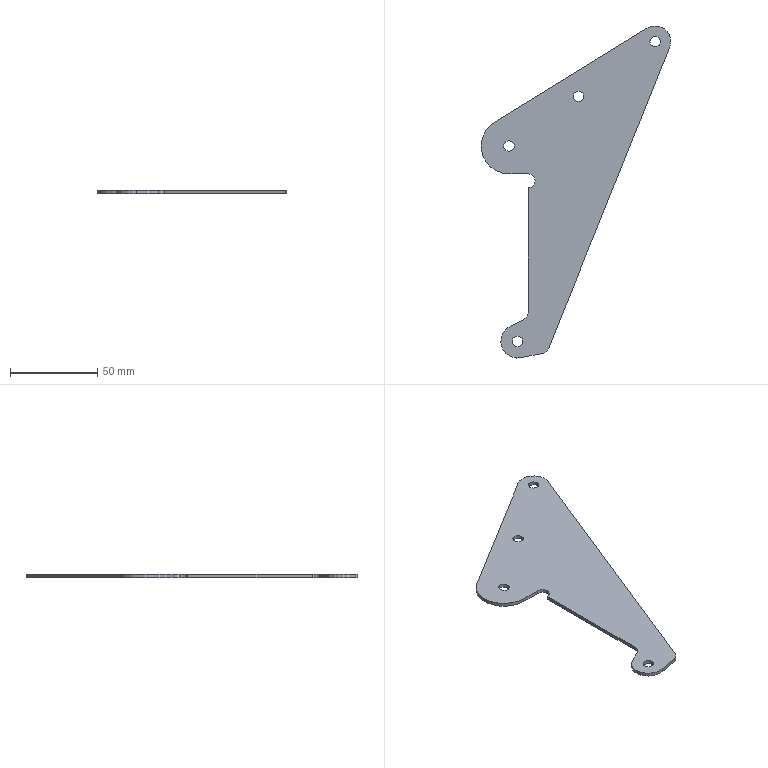Part | STEP file | 1 solid | 24 faces | box 109 x 190.824 x 2 mm | volume 17033 mm3 | cylinder 16 | plane 8 | commonest cylinder face diameters 6 x8 8 x2 10 x2 18 x2 19.149 x1 32 x1